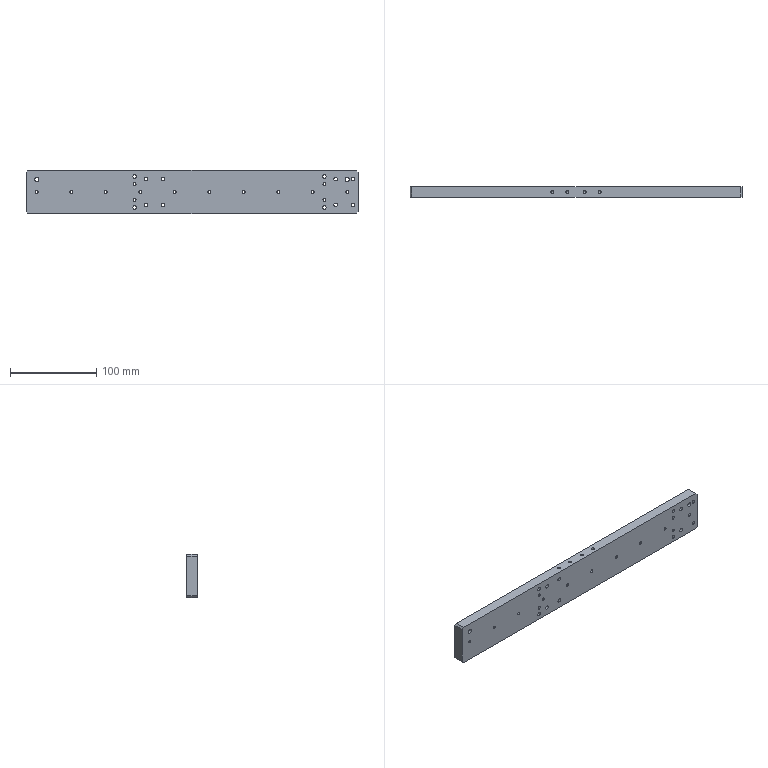CAM job | NX | 3+2 milling, drilling | part box 385 x 12 x 50 mm | stock box 390 x 15 x 55 mm
Tools:
number,name,description,diameter,corner_radius,flute_length,length,flutes
9,D10,平底铣刀-粗,10.0,0.0,35.0,75.0,2
7,D6-J,平底铣刀-精,6.0,0.0,25.0,75.0,2
1,D80R0.8飞刀,圆鼻刀-粗,80.0,0.8,50.0,75.0,2
1,D80R0.8飞刀-J,圆鼻刀-精,80.0,0.8,50.0,75.0,2
2,D6倒角刀,倒角刀,6.0,0.0,3.0,25.0,2
21,M4X0.7,丝锥,3.3,0.0,35.0,50.0,2
22,M5X0.8,丝锥,4.2,0.0,35.0,50.0,2
19,D4铰刀,Drilling Tool,4.0,0.0,75.0,100.0,6
20,D5铰刀,Drilling Tool,5.0,0.0,75.0,100.0,6
13,ZT3.4,钻头,3.4,0.0,35.0,50.0,2
17,ZT3.9,Drilling Tool,3.9,0.0,35.0,50.0,2
18,ZT4.9,Drilling Tool,4.9,0.0,35.0,50.0,2
14,ZT4.3,Drilling Tool,4.3,0.0,50.0,75.0,4
Operations:
program,operation,operation_type,tool,method,geometry_group,spindle_rpm,surface_speed,feed_per_tooth,feed_cut,feed_plunge,cut_length_mm,path_length_mm,cut_time_min,machine_time_min
B,底壁铣飞面一刀开粗_COPY,VolumeBased25DMillingOperation,D80R0.8飞刀,分层开粗-切深K-步距G,W-B,2800.0,703.696,0.5357,3000.0,100.0,2465.97,4611.947,0.822,1.037
B,底壁铣飞面一刀精光_COPY,VolumeBased25DMillingOperation,D80R0.8飞刀-J,侧刃精光-切深K-步距G,W-B,4000.0,1005.28,0.125,1000.0,100.0,492.998,588.998,0.493,0.5026
B,NG_钻倒角_3,Operation,D6倒角刀,METHOD,W-B,8000.0,150.796,0.0625,1000.0,0.0,72.8,692.847,0.0728,0.1348
B,NG_钻倒角_4,Operation,D6倒角刀,METHOD,W-B,8000.0,150.796,0.0625,1000.0,0.0,21.2,443.67,0.0212,0.0634
B,NG_钻倒角_5,Operation,D6倒角刀,METHOD,W-B,8000.0,150.796,0.0625,1000.0,0.0,11.6,486.212,0.0116,0.0591
B,NG_钻倒角_6,Operation,D6倒角刀,METHOD,W-B,8000.0,150.796,0.0625,1000.0,0.0,45.6,553.417,0.0456,0.0964
B,C0.3封闭铣廓倒角6X45L_COPY,PlanarMilling,D6倒角刀,爬面_倒角-切深0-步距G,W-B,7000.0,131.0,0.1071,1500.0,100.0,882.842,978.842,0.5886,0.5982
A,顶面,FaceMilling,D80R0.8飞刀,侧刃精光-切深K-步距G,W-A,4500.0,1385.0,0.1667,1500.0,100.0,479.0,575.0,0.3193,0.3289
A,外形粗_2,VolumeBased25DMillingOperation,D10,METHOD,W-A,8000.0,251.327,0.375,6000.0,80.0,15256.591,15367.091,2.543,2.554
A,打点-深0.8,Operation,D6倒角刀,NONE,W-A,8000.0,150.796,0.0312,500.0,90.0,50.4,793.801,0.1008,0.1751
A,通孔-M4螺纹底孔,Operation,ZT3.4,NONE,W-A,3000.0,31.102,0.05,300.0,90.0,266.0,1051.252,0.8867,0.9652
A,通孔-精孔4.0预钻,Operation,ZT3.9,NONE,W-A,3000.0,36.757,0.0417,250.0,90.0,68.503,532.037,0.274,0.3204
A,通孔-M5螺纹底孔,Operation,ZT4.3,NONE,W-A,3000.0,39.584,0.0583,350.0,90.0,160.0,767.136,0.4571,0.5179
A,通孔-精孔6.0预钻,Operation,ZT4.9,NONE,W-A,2500.0,38.484,0.05,250.0,90.0,34.829,530.659,0.1393,0.1889
A,仅选体,SurfaceContour,D6倒角刀,METHOD,W-A,8000.0,150.796,0.1875,3000.0,100.0,882.615,978.417,0.2942,0.3038
A,NG_钻倒角_1,Operation,D6倒角刀,METHOD,W-A,8000.0,150.796,0.0312,500.0,0.0,72.8,692.847,0.1456,0.2076
A,NG_钻倒角_2,Operation,D6倒角刀,METHOD,W-A,8000.0,150.796,0.0312,500.0,0.0,21.2,443.67,0.0424,0.0846
A,铣倒角_1,PlanarMilling,D6倒角刀,METHOD,W-A,8000.0,150.796,0.0312,500.0,100.0,144.163,1293.615,0.2883,0.4033
A,铣倒角_2,PlanarMilling,D6倒角刀,METHOD,W-A,8000.0,150.796,0.0312,500.0,100.0,36.963,600.532,0.0739,0.1303
A,REAM,Operation,D4铰刀,METHOD,W-A,500.0,6.283,0.0167,50.0,0.0,56.0,507.03,1.12,1.165
A,REAM_2,Operation,D5铰刀,METHOD,W-A,500.0,7.854,0.0167,50.0,0.0,28.0,517.001,0.56,0.6089
A,通孔-攻牙M4,Operation,M4X0.7,METHOD,W-A,600.0,6.22,0.0006,0.7,90.0,224.0,967.252,320.0,320.074
A,通孔-攻牙M5,Operation,M5X0.8,METHOD,W-A,500.0,6.597,0.0008,0.8,90.0,132.0,711.136,165.0,165.058
A,外形半精_2,VolumeBased25DMillingOperation,D6-J,METHOD,W-A,9000.0,169.646,0.0667,1200.0,100.0,889.08,1012.08,0.7409,0.7532